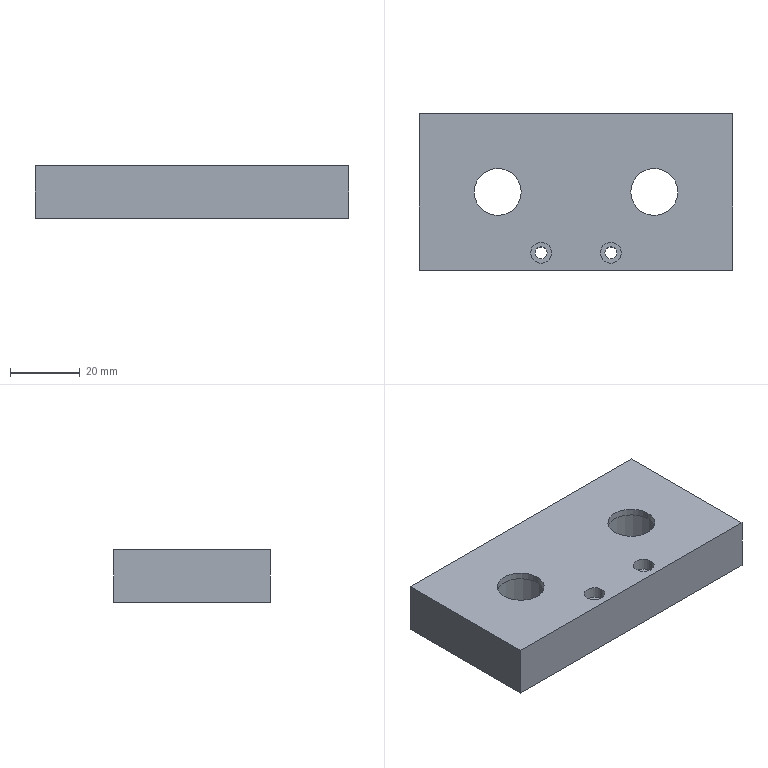Part | STEP file | X77-08308 | 1 solid | 26 faces | box 90 x 45 x 15 mm | volume 51606 mm3 | cylinder 16 | plane 10 | commonest cylinder face diameters 3.4 x4 6 x4 13.5 x4 20 x4
STEP:
#1=CARTESIAN_POINT('',(-591.701,750.64,11.6));
#2=VERTEX_POINT('',#1);
#3=CARTESIAN_POINT('',(-585.701,750.64,11.6));
#4=VERTEX_POINT('',#3);
#5=CARTESIAN_POINT('',(-588.701,750.64,11.6));
#6=DIRECTION('',(0.,0.,1.));
#7=DIRECTION('',(1.,0.,0.));
#8=AXIS2_PLACEMENT_3D('',#5,#6,#7);
#9=CIRCLE('',#8,3.);
#10=EDGE_CURVE('',#2,#4,#9,.T.);
#11=ORIENTED_EDGE('',*,*,#10,.F.);
#12=CARTESIAN_POINT('',(-591.701,750.64,15.));
#13=VERTEX_POINT('',#12);
#14=CARTESIAN_POINT('',(-591.701,750.64,15.));
#15=DIRECTION('',(0.,0.,1.));
#16=VECTOR('',#15,1000.);
#17=LINE('',#14,#16);
#18=EDGE_CURVE('',#2,#13,#17,.T.);
#19=ORIENTED_EDGE('',*,*,#18,.T.);
#20=CARTESIAN_POINT('',(-585.701,750.64,15.));
#21=VERTEX_POINT('',#20);
#22=CARTESIAN_POINT('',(-588.701,750.64,15.));
#23=DIRECTION('',(0.,0.,1.));
#24=DIRECTION('',(1.,0.,0.));
#25=AXIS2_PLACEMENT_3D('',#22,#23,#24);
#26=CIRCLE('',#25,3.);
#27=EDGE_CURVE('',#13,#21,#26,.T.);
#28=ORIENTED_EDGE('',*,*,#27,.T.);
#29=CARTESIAN_POINT('',(-585.701,750.64,15.));
#30=DIRECTION('',(0.,0.,1.));
#31=VECTOR('',#30,1000.);
#32=LINE('',#29,#31);
#33=EDGE_CURVE('',#4,#21,#32,.T.);
#34=ORIENTED_EDGE('',*,*,#33,.F.);
#35=EDGE_LOOP('',(#11,#19,#28,#34));
#36=FACE_OUTER_BOUND('',#35,.T.);
#37=CARTESIAN_POINT('',(-588.701,750.64,15.));
#38=DIRECTION('',(0.,0.,1.));
#39=DIRECTION('',(1.,0.,0.));
#40=AXIS2_PLACEMENT_3D('',#37,#38,#39);
#41=CYLINDRICAL_SURFACE('',#40,3.);
#42=ADVANCED_FACE('',(#36),#41,.F.);
#43=CARTESIAN_POINT('',(-590.401,750.64,0.));
#44=VERTEX_POINT('',#43);
#45=CARTESIAN_POINT('',(-587.001,750.64,0.));
#46=VERTEX_POINT('',#45);
#47=CARTESIAN_POINT('',(-588.701,750.64,0.));
#48=DIRECTION('',(0.,0.,1.));
#49=DIRECTION('',(1.,0.,0.));
#50=AXIS2_PLACEMENT_3D('',#47,#48,#49);
#51=CIRCLE('',#50,1.7);
#52=EDGE_CURVE('',#44,#46,#51,.T.);
#53=ORIENTED_EDGE('',*,*,#52,.F.);
#54=CARTESIAN_POINT('',(-590.401,750.64,11.6));
#55=VERTEX_POINT('',#54);
#56=CARTESIAN_POINT('',(-590.401,750.64,15.));
#57=DIRECTION('',(0.,0.,1.));
#58=VECTOR('',#57,1000.);
#59=LINE('',#56,#58);
#60=EDGE_CURVE('',#44,#55,#59,.T.);
#61=ORIENTED_EDGE('',*,*,#60,.T.);
#62=CARTESIAN_POINT('',(-587.001,750.64,11.6));
#63=VERTEX_POINT('',#62);
#64=CARTESIAN_POINT('',(-588.701,750.64,11.6));
#65=DIRECTION('',(0.,0.,1.));
#66=DIRECTION('',(1.,0.,0.));
#67=AXIS2_PLACEMENT_3D('',#64,#65,#66);
#68=CIRCLE('',#67,1.7);
#69=EDGE_CURVE('',#55,#63,#68,.T.);
#70=ORIENTED_EDGE('',*,*,#69,.T.);
#71=CARTESIAN_POINT('',(-587.001,750.64,15.));
#72=DIRECTION('',(0.,0.,1.));
#73=VECTOR('',#72,1000.);
#74=LINE('',#71,#73);
#75=EDGE_CURVE('',#46,#63,#74,.T.);
#76=ORIENTED_EDGE('',*,*,#75,.F.);
#77=EDGE_LOOP('',(#53,#61,#70,#76));
#78=FACE_OUTER_BOUND('',#77,.T.);
#79=CARTESIAN_POINT('',(-588.701,750.64,15.));
#80=DIRECTION('',(0.,0.,1.));
#81=DIRECTION('',(1.,0.,0.));
#82=AXIS2_PLACEMENT_3D('',#79,#80,#81);
#83=CYLINDRICAL_SURFACE('',#82,1.7);
#84=ADVANCED_FACE('',(#78),#83,.F.);
#85=CARTESIAN_POINT('',(-571.701,750.64,11.6));
#86=VERTEX_POINT('',#85);
#87=CARTESIAN_POINT('',(-565.701,750.64,11.6));
#88=VERTEX_POINT('',#87);
#89=CARTESIAN_POINT('',(-568.701,750.64,11.6));
#90=DIRECTION('',(0.,0.,1.));
#91=DIRECTION('',(1.,0.,0.));
#92=AXIS2_PLACEMENT_3D('',#89,#90,#91);
#93=CIRCLE('',#92,3.);
#94=EDGE_CURVE('',#86,#88,#93,.T.);
#95=ORIENTED_EDGE('',*,*,#94,.F.);
#96=CARTESIAN_POINT('',(-571.701,750.64,15.));
#97=VERTEX_POINT('',#96);
#98=CARTESIAN_POINT('',(-571.701,750.64,15.));
#99=DIRECTION('',(0.,0.,1.));
#100=VECTOR('',#99,1000.);
#101=LINE('',#98,#100);
#102=EDGE_CURVE('',#86,#97,#101,.T.);
#103=ORIENTED_EDGE('',*,*,#102,.T.);
#104=CARTESIAN_POINT('',(-565.701,750.64,15.));
#105=VERTEX_POINT('',#104);
#106=CARTESIAN_POINT('',(-568.701,750.64,15.));
#107=DIRECTION('',(0.,0.,1.));
#108=DIRECTION('',(1.,0.,0.));
#109=AXIS2_PLACEMENT_3D('',#106,#107,#108);
#110=CIRCLE('',#109,3.);
#111=EDGE_CURVE('',#97,#105,#110,.T.);
#112=ORIENTED_EDGE('',*,*,#111,.T.);
#113=CARTESIAN_POINT('',(-565.701,750.64,15.));
#114=DIRECTION('',(0.,0.,1.));
#115=VECTOR('',#114,1000.);
#116=LINE('',#113,#115);
#117=EDGE_CURVE('',#88,#105,#116,.T.);
#118=ORIENTED_EDGE('',*,*,#117,.F.);
#119=EDGE_LOOP('',(#95,#103,#112,#118));
#120=FACE_OUTER_BOUND('',#119,.T.);
#121=CARTESIAN_POINT('',(-568.701,750.64,15.));
#122=DIRECTION('',(0.,0.,1.));
#123=DIRECTION('',(1.,0.,0.));
#124=AXIS2_PLACEMENT_3D('',#121,#122,#123);
#125=CYLINDRICAL_SURFACE('',#124,3.);
#126=ADVANCED_FACE('',(#120),#125,.F.);
#127=CARTESIAN_POINT('',(-570.401,750.64,0.));
#128=VERTEX_POINT('',#127);
#129=CARTESIAN_POINT('',(-567.001,750.64,0.));
#130=VERTEX_POINT('',#129);
#131=CARTESIAN_POINT('',(-568.701,750.64,0.));
#132=DIRECTION('',(0.,0.,1.));
#133=DIRECTION('',(1.,0.,0.));
#134=AXIS2_PLACEMENT_3D('',#131,#132,#133);
#135=CIRCLE('',#134,1.7);
#136=EDGE_CURVE('',#128,#130,#135,.T.);
#137=ORIENTED_EDGE('',*,*,#136,.F.);
#138=CARTESIAN_POINT('',(-570.401,750.64,11.6));
#139=VERTEX_POINT('',#138);
#140=CARTESIAN_POINT('',(-570.401,750.64,15.));
#141=DIRECTION('',(0.,0.,1.));
#142=VECTOR('',#141,1000.);
#143=LINE('',#140,#142);
#144=EDGE_CURVE('',#128,#139,#143,.T.);
#145=ORIENTED_EDGE('',*,*,#144,.T.);
#146=CARTESIAN_POINT('',(-567.001,750.64,11.6));
#147=VERTEX_POINT('',#146);
#148=CARTESIAN_POINT('',(-568.701,750.64,11.6));
#149=DIRECTION('',(0.,0.,1.));
#150=DIRECTION('',(1.,0.,0.));
#151=AXIS2_PLACEMENT_3D('',#148,#149,#150);
#152=CIRCLE('',#151,1.7);
#153=EDGE_CURVE('',#139,#147,#152,.T.);
#154=ORIENTED_EDGE('',*,*,#153,.T.);
#155=CARTESIAN_POINT('',(-567.001,750.64,15.));
#156=DIRECTION('',(0.,0.,1.));
#157=VECTOR('',#156,1000.);
#158=LINE('',#155,#157);
#159=EDGE_CURVE('',#130,#147,#158,.T.);
#160=ORIENTED_EDGE('',*,*,#159,.F.);
#161=EDGE_LOOP('',(#137,#145,#154,#160));
#162=FACE_OUTER_BOUND('',#161,.T.);
#163=CARTESIAN_POINT('',(-568.701,750.64,15.));
#164=DIRECTION('',(0.,0.,1.));
#165=DIRECTION('',(1.,0.,0.));
#166=AXIS2_PLACEMENT_3D('',#163,#164,#165);
#167=CYLINDRICAL_SURFACE('',#166,1.7);
#168=ADVANCED_FACE('',(#162),#167,.F.);
#169=CARTESIAN_POINT('',(-546.201,768.14,13.));
#170=VERTEX_POINT('',#169);
#171=CARTESIAN_POINT('',(-566.201,768.14,13.));
#172=VERTEX_POINT('',#171);
#173=CARTESIAN_POINT('',(-556.201,768.14,13.));
#174=DIRECTION('',(0.,0.,-1.));
#175=DIRECTION('',(-1.,0.,0.));
#176=AXIS2_PLACEMENT_3D('',#173,#174,#175);
#177=CIRCLE('',#176,10.);
#178=EDGE_CURVE('',#170,#172,#177,.T.);
#179=ORIENTED_EDGE('',*,*,#178,.F.);
#180=CARTESIAN_POINT('',(-546.201,768.14,0.));
#181=VERTEX_POINT('',#180);
#182=CARTESIAN_POINT('',(-546.201,768.14,0.));
#183=DIRECTION('',(0.,0.,-1.));
#184=VECTOR('',#183,1000.);
#185=LINE('',#182,#184);
#186=EDGE_CURVE('',#170,#181,#185,.T.);
#187=ORIENTED_EDGE('',*,*,#186,.T.);
#188=CARTESIAN_POINT('',(-566.201,768.14,0.));
#189=VERTEX_POINT('',#188);
#190=CARTESIAN_POINT('',(-556.201,768.14,0.));
#191=DIRECTION('',(0.,0.,-1.));
#192=DIRECTION('',(-1.,0.,0.));
#193=AXIS2_PLACEMENT_3D('',#190,#191,#192);
#194=CIRCLE('',#193,10.);
#195=EDGE_CURVE('',#181,#189,#194,.T.);
#196=ORIENTED_EDGE('',*,*,#195,.T.);
#197=CARTESIAN_POINT('',(-566.201,768.14,0.));
#198=DIRECTION('',(0.,0.,-1.));
#199=VECTOR('',#198,1000.);
#200=LINE('',#197,#199);
#201=EDGE_CURVE('',#172,#189,#200,.T.);
#202=ORIENTED_EDGE('',*,*,#201,.F.);
#203=EDGE_LOOP('',(#179,#187,#196,#202));
#204=FACE_OUTER_BOUND('',#203,.T.);
#205=CARTESIAN_POINT('',(-556.201,768.14,0.));
#206=DIRECTION('',(0.,0.,-1.));
#207=DIRECTION('',(-1.,0.,0.));
#208=AXIS2_PLACEMENT_3D('',#205,#206,#207);
#209=CYLINDRICAL_SURFACE('',#208,10.);
#210=ADVANCED_FACE('',(#204),#209,.F.);
#211=CARTESIAN_POINT('',(-549.451,768.14,15.));
#212=VERTEX_POINT('',#211);
#213=CARTESIAN_POINT('',(-562.951,768.14,15.));
#214=VERTEX_POINT('',#213);
#215=CARTESIAN_POINT('',(-556.201,768.14,15.));
#216=DIRECTION('',(0.,0.,-1.));
#217=DIRECTION('',(-1.,0.,0.));
#218=AXIS2_PLACEMENT_3D('',#215,#216,#217);
#219=CIRCLE('',#218,6.75);
#220=EDGE_CURVE('',#212,#214,#219,.T.);
#221=ORIENTED_EDGE('',*,*,#220,.F.);
#222=CARTESIAN_POINT('',(-549.451,768.14,13.));
#223=VERTEX_POINT('',#222);
#224=CARTESIAN_POINT('',(-549.451,768.14,0.));
#225=DIRECTION('',(0.,0.,-1.));
#226=VECTOR('',#225,1000.);
#227=LINE('',#224,#226);
#228=EDGE_CURVE('',#212,#223,#227,.T.);
#229=ORIENTED_EDGE('',*,*,#228,.T.);
#230=CARTESIAN_POINT('',(-562.951,768.14,13.));
#231=VERTEX_POINT('',#230);
#232=CARTESIAN_POINT('',(-556.201,768.14,13.));
#233=DIRECTION('',(0.,0.,-1.));
#234=DIRECTION('',(-1.,0.,0.));
#235=AXIS2_PLACEMENT_3D('',#232,#233,#234);
#236=CIRCLE('',#235,6.75);
#237=EDGE_CURVE('',#223,#231,#236,.T.);
#238=ORIENTED_EDGE('',*,*,#237,.T.);
#239=CARTESIAN_POINT('',(-562.951,768.14,0.));
#240=DIRECTION('',(0.,0.,-1.));
#241=VECTOR('',#240,1000.);
#242=LINE('',#239,#241);
#243=EDGE_CURVE('',#214,#231,#242,.T.);
#244=ORIENTED_EDGE('',*,*,#243,.F.);
#245=EDGE_LOOP('',(#221,#229,#238,#244));
#246=FACE_OUTER_BOUND('',#245,.T.);
#247=CARTESIAN_POINT('',(-556.201,768.14,0.));
#248=DIRECTION('',(0.,0.,-1.));
#249=DIRECTION('',(-1.,0.,0.));
#250=AXIS2_PLACEMENT_3D('',#247,#248,#249);
#251=CYLINDRICAL_SURFACE('',#250,6.75);
#252=ADVANCED_FACE('',(#246),#251,.F.);
#253=CARTESIAN_POINT('',(-591.201,768.14,13.));
#254=VERTEX_POINT('',#253);
#255=CARTESIAN_POINT('',(-611.201,768.14,13.));
#256=VERTEX_POINT('',#255);
#257=CARTESIAN_POINT('',(-601.201,768.14,13.));
#258=DIRECTION('',(0.,0.,-1.));
#259=DIRECTION('',(-1.,0.,0.));
#260=AXIS2_PLACEMENT_3D('',#257,#258,#259);
#261=CIRCLE('',#260,10.);
#262=EDGE_CURVE('',#254,#256,#261,.T.);
#263=ORIENTED_EDGE('',*,*,#262,.F.);
#264=CARTESIAN_POINT('',(-591.201,768.14,0.));
#265=VERTEX_POINT('',#264);
#266=CARTESIAN_POINT('',(-591.201,768.14,0.));
#267=DIRECTION('',(0.,0.,-1.));
#268=VECTOR('',#267,1000.);
#269=LINE('',#266,#268);
#270=EDGE_CURVE('',#254,#265,#269,.T.);
#271=ORIENTED_EDGE('',*,*,#270,.T.);
#272=CARTESIAN_POINT('',(-611.201,768.14,0.));
#273=VERTEX_POINT('',#272);
#274=CARTESIAN_POINT('',(-601.201,768.14,0.));
#275=DIRECTION('',(0.,0.,-1.));
#276=DIRECTION('',(-1.,0.,0.));
#277=AXIS2_PLACEMENT_3D('',#274,#275,#276);
#278=CIRCLE('',#277,10.);
#279=EDGE_CURVE('',#265,#273,#278,.T.);
#280=ORIENTED_EDGE('',*,*,#279,.T.);
#281=CARTESIAN_POINT('',(-611.201,768.14,0.));
#282=DIRECTION('',(0.,0.,-1.));
#283=VECTOR('',#282,1000.);
#284=LINE('',#281,#283);
#285=EDGE_CURVE('',#256,#273,#284,.T.);
#286=ORIENTED_EDGE('',*,*,#285,.F.);
#287=EDGE_LOOP('',(#263,#271,#280,#286));
#288=FACE_OUTER_BOUND('',#287,.T.);
#289=CARTESIAN_POINT('',(-601.201,768.14,0.));
#290=DIRECTION('',(0.,0.,-1.));
#291=DIRECTION('',(-1.,0.,0.));
#292=AXIS2_PLACEMENT_3D('',#289,#290,#291);
#293=CYLINDRICAL_SURFACE('',#292,10.);
#294=ADVANCED_FACE('',(#288),#293,.F.);
#295=CARTESIAN_POINT('',(-594.451,768.14,15.));
#296=VERTEX_POINT('',#295);
#297=CARTESIAN_POINT('',(-607.951,768.14,15.));
#298=VERTEX_POINT('',#297);
#299=CARTESIAN_POINT('',(-601.201,768.14,15.));
#300=DIRECTION('',(0.,0.,-1.));
#301=DIRECTION('',(-1.,0.,0.));
#302=AXIS2_PLACEMENT_3D('',#299,#300,#301);
#303=CIRCLE('',#302,6.75);
#304=EDGE_CURVE('',#296,#298,#303,.T.);
#305=ORIENTED_EDGE('',*,*,#304,.F.);
#306=CARTESIAN_POINT('',(-594.451,768.14,13.));
#307=VERTEX_POINT('',#306);
#308=CARTESIAN_POINT('',(-594.451,768.14,0.));
#309=DIRECTION('',(0.,0.,-1.));
#310=VECTOR('',#309,1000.);
#311=LINE('',#308,#310);
#312=EDGE_CURVE('',#296,#307,#311,.T.);
#313=ORIENTED_EDGE('',*,*,#312,.T.);
#314=CARTESIAN_POINT('',(-607.951,768.14,13.));
#315=VERTEX_POINT('',#314);
#316=CARTESIAN_POINT('',(-601.201,768.14,13.));
#317=DIRECTION('',(0.,0.,-1.));
#318=DIRECTION('',(-1.,0.,0.));
#319=AXIS2_PLACEMENT_3D('',#316,#317,#318);
#320=CIRCLE('',#319,6.75);
#321=EDGE_CURVE('',#307,#315,#320,.T.);
#322=ORIENTED_EDGE('',*,*,#321,.T.);
#323=CARTESIAN_POINT('',(-607.951,768.14,0.));
#324=DIRECTION('',(0.,0.,-1.));
#325=VECTOR('',#324,1000.);
#326=LINE('',#323,#325);
#327=EDGE_CURVE('',#298,#315,#326,.T.);
#328=ORIENTED_EDGE('',*,*,#327,.F.);
#329=EDGE_LOOP('',(#305,#313,#322,#328));
#330=FACE_OUTER_BOUND('',#329,.T.);
#331=CARTESIAN_POINT('',(-601.201,768.14,0.));
#332=DIRECTION('',(0.,0.,-1.));
#333=DIRECTION('',(-1.,0.,0.));
#334=AXIS2_PLACEMENT_3D('',#331,#332,#333);
#335=CYLINDRICAL_SURFACE('',#334,6.75);
#336=ADVANCED_FACE('',(#330),#335,.F.);
#337=CARTESIAN_POINT('',(-623.701,790.64,0.));
#338=VERTEX_POINT('',#337);
#339=CARTESIAN_POINT('',(-623.701,745.64,0.));
#340=VERTEX_POINT('',#339);
#341=CARTESIAN_POINT('',(-623.701,790.64,0.));
#342=DIRECTION('',(0.,-1.,0.));
#343=VECTOR('',#342,1000.);
#344=LINE('',#341,#343);
#345=EDGE_CURVE('',#338,#340,#344,.T.);
#346=ORIENTED_EDGE('',*,*,#345,.T.);
#347=CARTESIAN_POINT('',(-623.701,745.64,15.));
#348=VERTEX_POINT('',#347);
#349=CARTESIAN_POINT('',(-623.701,745.64,15.));
#350=DIRECTION('',(0.,0.,-1.));
#351=VECTOR('',#350,1000.);
#352=LINE('',#349,#351);
#353=EDGE_CURVE('',#348,#340,#352,.T.);
#354=ORIENTED_EDGE('',*,*,#353,.F.);
#355=CARTESIAN_POINT('',(-623.701,790.64,15.));
#356=VERTEX_POINT('',#355);
#357=CARTESIAN_POINT('',(-623.701,790.64,15.));
#358=DIRECTION('',(0.,-1.,0.));
#359=VECTOR('',#358,1000.);
#360=LINE('',#357,#359);
#361=EDGE_CURVE('',#356,#348,#360,.T.);
#362=ORIENTED_EDGE('',*,*,#361,.F.);
#363=CARTESIAN_POINT('',(-623.701,790.64,15.));
#364=DIRECTION('',(0.,0.,-1.));
#365=VECTOR('',#364,1000.);
#366=LINE('',#363,#365);
#367=EDGE_CURVE('',#356,#338,#366,.T.);
#368=ORIENTED_EDGE('',*,*,#367,.T.);
#369=EDGE_LOOP('',(#346,#354,#362,#368));
#370=FACE_OUTER_BOUND('',#369,.T.);
#371=CARTESIAN_POINT('',(-623.701,790.64,15.));
#372=DIRECTION('',(1.,0.,0.));
#373=DIRECTION('',(0.,0.,-1.));
#374=AXIS2_PLACEMENT_3D('',#371,#372,#373);
#375=PLANE('',#374);
#376=ADVANCED_FACE('',(#370),#375,.F.);
#377=CARTESIAN_POINT('',(-533.701,745.64,0.));
#378=VERTEX_POINT('',#377);
#379=CARTESIAN_POINT('',(-623.701,745.64,0.));
#380=DIRECTION('',(1.,0.,0.));
#381=VECTOR('',#380,1000.);
#382=LINE('',#379,#381);
#383=EDGE_CURVE('',#340,#378,#382,.T.);
#384=ORIENTED_EDGE('',*,*,#383,.T.);
#385=CARTESIAN_POINT('',(-533.701,745.64,15.));
#386=VERTEX_POINT('',#385);
#387=CARTESIAN_POINT('',(-533.701,745.64,15.));
#388=DIRECTION('',(0.,0.,-1.));
#389=VECTOR('',#388,1000.);
#390=LINE('',#387,#389);
#391=EDGE_CURVE('',#386,#378,#390,.T.);
#392=ORIENTED_EDGE('',*,*,#391,.F.);
#393=CARTESIAN_POINT('',(-623.701,745.64,15.));
#394=DIRECTION('',(1.,0.,0.));
#395=VECTOR('',#394,1000.);
#396=LINE('',#393,#395);
#397=EDGE_CURVE('',#348,#386,#396,.T.);
#398=ORIENTED_EDGE('',*,*,#397,.F.);
#399=ORIENTED_EDGE('',*,*,#353,.T.);
#400=EDGE_LOOP('',(#384,#392,#398,#399));
#401=FACE_OUTER_BOUND('',#400,.T.);
#402=CARTESIAN_POINT('',(-623.701,745.64,15.));
#403=DIRECTION('',(0.,1.,0.));
#404=DIRECTION('',(0.,0.,1.));
#405=AXIS2_PLACEMENT_3D('',#402,#403,#404);
#406=PLANE('',#405);
#407=ADVANCED_FACE('',(#401),#406,.F.);
#408=CARTESIAN_POINT('',(-533.701,790.64,0.));
#409=VERTEX_POINT('',#408);
#410=CARTESIAN_POINT('',(-533.701,790.64,0.));
#411=DIRECTION('',(0.,1.,0.));
#412=VECTOR('',#411,1000.);
#413=LINE('',#410,#412);
#414=EDGE_CURVE('',#378,#409,#413,.T.);
#415=ORIENTED_EDGE('',*,*,#414,.T.);
#416=CARTESIAN_POINT('',(-533.701,790.64,15.));
#417=VERTEX_POINT('',#416);
#418=CARTESIAN_POINT('',(-533.701,790.64,15.));
#419=DIRECTION('',(0.,0.,-1.));
#420=VECTOR('',#419,1000.);
#421=LINE('',#418,#420);
#422=EDGE_CURVE('',#417,#409,#421,.T.);
#423=ORIENTED_EDGE('',*,*,#422,.F.);
#424=CARTESIAN_POINT('',(-533.701,790.64,15.));
#425=DIRECTION('',(0.,1.,0.));
#426=VECTOR('',#425,1000.);
#427=LINE('',#424,#426);
#428=EDGE_CURVE('',#386,#417,#427,.T.);
#429=ORIENTED_EDGE('',*,*,#428,.F.);
#430=ORIENTED_EDGE('',*,*,#391,.T.);
#431=EDGE_LOOP('',(#415,#423,#429,#430));
#432=FACE_OUTER_BOUND('',#431,.T.);
#433=CARTESIAN_POINT('',(-533.701,790.64,15.));
#434=DIRECTION('',(-1.,0.,0.));
#435=DIRECTION('',(0.,0.,1.));
#436=AXIS2_PLACEMENT_3D('',#433,#434,#435);
#437=PLANE('',#436);
#438=ADVANCED_FACE('',(#432),#437,.F.);
#439=CARTESIAN_POINT('',(-623.701,790.64,0.));
#440=DIRECTION('',(-1.,0.,0.));
#441=VECTOR('',#440,1000.);
#442=LINE('',#439,#441);
#443=EDGE_CURVE('',#409,#338,#442,.T.);
#444=ORIENTED_EDGE('',*,*,#443,.T.);
#445=ORIENTED_EDGE('',*,*,#367,.F.);
#446=CARTESIAN_POINT('',(-623.701,790.64,15.));
#447=DIRECTION('',(-1.,0.,0.));
#448=VECTOR('',#447,1000.);
#449=LINE('',#446,#448);
#450=EDGE_CURVE('',#417,#356,#449,.T.);
#451=ORIENTED_EDGE('',*,*,#450,.F.);
#452=ORIENTED_EDGE('',*,*,#422,.T.);
#453=EDGE_LOOP('',(#444,#445,#451,#452));
#454=FACE_OUTER_BOUND('',#453,.T.);
#455=CARTESIAN_POINT('',(-623.701,790.64,15.));
#456=DIRECTION('',(0.,-1.,0.));
#457=DIRECTION('',(0.,0.,-1.));
#458=AXIS2_PLACEMENT_3D('',#455,#456,#457);
#459=PLANE('',#458);
#460=ADVANCED_FACE('',(#454),#459,.F.);
#461=CARTESIAN_POINT('',(-588.701,750.64,15.));
#462=DIRECTION('',(0.,0.,1.));
#463=DIRECTION('',(1.,0.,0.));
#464=AXIS2_PLACEMENT_3D('',#461,#462,#463);
#465=CIRCLE('',#464,3.);
#466=EDGE_CURVE('',#21,#13,#465,.T.);
#467=ORIENTED_EDGE('',*,*,#466,.F.);
#468=ORIENTED_EDGE('',*,*,#27,.F.);
#469=EDGE_LOOP('',(#467,#468));
#470=FACE_BOUND('',#469,.T.);
#471=CARTESIAN_POINT('',(-568.701,750.64,15.));
#472=DIRECTION('',(0.,0.,1.));
#473=DIRECTION('',(1.,0.,0.));
#474=AXIS2_PLACEMENT_3D('',#471,#472,#473);
#475=CIRCLE('',#474,3.);
#476=EDGE_CURVE('',#105,#97,#475,.T.);
#477=ORIENTED_EDGE('',*,*,#476,.F.);
#478=ORIENTED_EDGE('',*,*,#111,.F.);
#479=EDGE_LOOP('',(#477,#478));
#480=FACE_BOUND('',#479,.T.);
#481=CARTESIAN_POINT('',(-556.201,768.14,15.));
#482=DIRECTION('',(0.,0.,-1.));
#483=DIRECTION('',(-1.,0.,0.));
#484=AXIS2_PLACEMENT_3D('',#481,#482,#483);
#485=CIRCLE('',#484,6.75);
#486=EDGE_CURVE('',#214,#212,#485,.T.);
#487=ORIENTED_EDGE('',*,*,#486,.T.);
#488=ORIENTED_EDGE('',*,*,#220,.T.);
#489=EDGE_LOOP('',(#487,#488));
#490=FACE_BOUND('',#489,.T.);
#491=CARTESIAN_POINT('',(-601.201,768.14,15.));
#492=DIRECTION('',(0.,0.,-1.));
#493=DIRECTION('',(-1.,0.,0.));
#494=AXIS2_PLACEMENT_3D('',#491,#492,#493);
#495=CIRCLE('',#494,6.75);
#496=EDGE_CURVE('',#298,#296,#495,.T.);
#497=ORIENTED_EDGE('',*,*,#496,.T.);
#498=ORIENTED_EDGE('',*,*,#304,.T.);
#499=EDGE_LOOP('',(#497,#498));
#500=FACE_BOUND('',#499,.T.);
#501=ORIENTED_EDGE('',*,*,#361,.T.);
#502=ORIENTED_EDGE('',*,*,#397,.T.);
#503=ORIENTED_EDGE('',*,*,#428,.T.);
#504=ORIENTED_EDGE('',*,*,#450,.T.);
#505=EDGE_LOOP('',(#501,#502,#503,#504));
#506=FACE_OUTER_BOUND('',#505,.T.);
#507=CARTESIAN_POINT('',(-623.701,745.64,15.));
#508=DIRECTION('',(0.,0.,1.));
#509=DIRECTION('',(1.,0.,0.));
#510=AXIS2_PLACEMENT_3D('',#507,#508,#509);
#511=PLANE('',#510);
#512=ADVANCED_FACE('',(#470,#480,#490,#500,#506),#511,.T.);
#513=CARTESIAN_POINT('',(-588.701,750.64,0.));
#514=DIRECTION('',(0.,0.,1.));
#515=DIRECTION('',(1.,0.,0.));
#516=AXIS2_PLACEMENT_3D('',#513,#514,#515);
#517=CIRCLE('',#516,1.7);
#518=EDGE_CURVE('',#46,#44,#517,.T.);
#519=ORIENTED_EDGE('',*,*,#518,.T.);
#520=ORIENTED_EDGE('',*,*,#52,.T.);
#521=EDGE_LOOP('',(#519,#520));
#522=FACE_BOUND('',#521,.T.);
#523=CARTESIAN_POINT('',(-568.701,750.64,0.));
#524=DIRECTION('',(0.,0.,1.));
#525=DIRECTION('',(1.,0.,0.));
#526=AXIS2_PLACEMENT_3D('',#523,#524,#525);
#527=CIRCLE('',#526,1.7);
#528=EDGE_CURVE('',#130,#128,#527,.T.);
#529=ORIENTED_EDGE('',*,*,#528,.T.);
#530=ORIENTED_EDGE('',*,*,#136,.T.);
#531=EDGE_LOOP('',(#529,#530));
#532=FACE_BOUND('',#531,.T.);
#533=CARTESIAN_POINT('',(-556.201,768.14,0.));
#534=DIRECTION('',(0.,0.,-1.));
#535=DIRECTION('',(-1.,0.,0.));
#536=AXIS2_PLACEMENT_3D('',#533,#534,#535);
#537=CIRCLE('',#536,10.);
#538=EDGE_CURVE('',#189,#181,#537,.T.);
#539=ORIENTED_EDGE('',*,*,#538,.F.);
#540=ORIENTED_EDGE('',*,*,#195,.F.);
#541=EDGE_LOOP('',(#539,#540));
#542=FACE_BOUND('',#541,.T.);
#543=CARTESIAN_POINT('',(-601.201,768.14,0.));
#544=DIRECTION('',(0.,0.,-1.));
#545=DIRECTION('',(-1.,0.,0.));
#546=AXIS2_PLACEMENT_3D('',#543,#544,#545);
#547=CIRCLE('',#546,10.);
#548=EDGE_CURVE('',#273,#265,#547,.T.);
#549=ORIENTED_EDGE('',*,*,#548,.F.);
#550=ORIENTED_EDGE('',*,*,#279,.F.);
#551=EDGE_LOOP('',(#549,#550));
#552=FACE_BOUND('',#551,.T.);
#553=ORIENTED_EDGE('',*,*,#345,.F.);
#554=ORIENTED_EDGE('',*,*,#443,.F.);
#555=ORIENTED_EDGE('',*,*,#414,.F.);
#556=ORIENTED_EDGE('',*,*,#383,.F.);
#557=EDGE_LOOP('',(#553,#554,#555,#556));
#558=FACE_OUTER_BOUND('',#557,.T.);
#559=CARTESIAN_POINT('',(-623.701,745.64,0.));
#560=DIRECTION('',(0.,0.,1.));
#561=DIRECTION('',(1.,0.,0.));
#562=AXIS2_PLACEMENT_3D('',#559,#560,#561);
#563=PLANE('',#562);
#564=ADVANCED_FACE('',(#522,#532,#542,#552,#558),#563,.F.);
#565=ORIENTED_EDGE('',*,*,#312,.F.);
#566=ORIENTED_EDGE('',*,*,#496,.F.);
#567=ORIENTED_EDGE('',*,*,#327,.T.);
#568=CARTESIAN_POINT('',(-601.201,768.14,13.));
#569=DIRECTION('',(0.,0.,-1.));
#570=DIRECTION('',(-1.,0.,0.));
#571=AXIS2_PLACEMENT_3D('',#568,#569,#570);
#572=CIRCLE('',#571,6.75);
#573=EDGE_CURVE('',#315,#307,#572,.T.);
#574=ORIENTED_EDGE('',*,*,#573,.T.);
#575=EDGE_LOOP('',(#565,#566,#567,#574));
#576=FACE_OUTER_BOUND('',#575,.T.);
#577=CARTESIAN_POINT('',(-601.201,768.14,0.));
#578=DIRECTION('',(0.,0.,-1.));
#579=DIRECTION('',(-1.,0.,0.));
#580=AXIS2_PLACEMENT_3D('',#577,#578,#579);
#581=CYLINDRICAL_SURFACE('',#580,6.75);
#582=ADVANCED_FACE('',(#576),#581,.F.);
#583=ORIENTED_EDGE('',*,*,#573,.F.);
#584=ORIENTED_EDGE('',*,*,#321,.F.);
#585=EDGE_LOOP('',(#583,#584));
#586=FACE_BOUND('',#585,.T.);
#587=CARTESIAN_POINT('',(-601.201,768.14,13.));
#588=DIRECTION('',(0.,0.,-1.));
#589=DIRECTION('',(-1.,0.,0.));
#590=AXIS2_PLACEMENT_3D('',#587,#588,#589);
#591=CIRCLE('',#590,10.);
#592=EDGE_CURVE('',#256,#254,#591,.T.);
#593=ORIENTED_EDGE('',*,*,#592,.T.);
#594=ORIENTED_EDGE('',*,*,#262,.T.);
#595=EDGE_LOOP('',(#593,#594));
#596=FACE_OUTER_BOUND('',#595,.T.);
#597=CARTESIAN_POINT('',(-594.451,768.14,13.));
#598=DIRECTION('',(0.,0.,1.));
#599=DIRECTION('',(1.,0.,0.));
#600=AXIS2_PLACEMENT_3D('',#597,#598,#599);
#601=PLANE('',#600);
#602=ADVANCED_FACE('',(#586,#596),#601,.F.);
#603=ORIENTED_EDGE('',*,*,#270,.F.);
#604=ORIENTED_EDGE('',*,*,#592,.F.);
#605=ORIENTED_EDGE('',*,*,#285,.T.);
#606=ORIENTED_EDGE('',*,*,#548,.T.);
#607=EDGE_LOOP('',(#603,#604,#605,#606));
#608=FACE_OUTER_BOUND('',#607,.T.);
#609=CARTESIAN_POINT('',(-601.201,768.14,0.));
#610=DIRECTION('',(0.,0.,-1.));
#611=DIRECTION('',(-1.,0.,0.));
#612=AXIS2_PLACEMENT_3D('',#609,#610,#611);
#613=CYLINDRICAL_SURFACE('',#612,10.);
#614=ADVANCED_FACE('',(#608),#613,.F.);
#615=ORIENTED_EDGE('',*,*,#228,.F.);
#616=ORIENTED_EDGE('',*,*,#486,.F.);
#617=ORIENTED_EDGE('',*,*,#243,.T.);
#618=CARTESIAN_POINT('',(-556.201,768.14,13.));
#619=DIRECTION('',(0.,0.,-1.));
#620=DIRECTION('',(-1.,0.,0.));
#621=AXIS2_PLACEMENT_3D('',#618,#619,#620);
#622=CIRCLE('',#621,6.75);
#623=EDGE_CURVE('',#231,#223,#622,.T.);
#624=ORIENTED_EDGE('',*,*,#623,.T.);
#625=EDGE_LOOP('',(#615,#616,#617,#624));
#626=FACE_OUTER_BOUND('',#625,.T.);
#627=CARTESIAN_POINT('',(-556.201,768.14,0.));
#628=DIRECTION('',(0.,0.,-1.));
#629=DIRECTION('',(-1.,0.,0.));
#630=AXIS2_PLACEMENT_3D('',#627,#628,#629);
#631=CYLINDRICAL_SURFACE('',#630,6.75);
#632=ADVANCED_FACE('',(#626),#631,.F.);
#633=ORIENTED_EDGE('',*,*,#623,.F.);
#634=ORIENTED_EDGE('',*,*,#237,.F.);
#635=EDGE_LOOP('',(#633,#634));
#636=FACE_BOUND('',#635,.T.);
#637=CARTESIAN_POINT('',(-556.201,768.14,13.));
#638=DIRECTION('',(0.,0.,-1.));
#639=DIRECTION('',(-1.,0.,0.));
#640=AXIS2_PLACEMENT_3D('',#637,#638,#639);
#641=CIRCLE('',#640,10.);
#642=EDGE_CURVE('',#172,#170,#641,.T.);
#643=ORIENTED_EDGE('',*,*,#642,.T.);
#644=ORIENTED_EDGE('',*,*,#178,.T.);
#645=EDGE_LOOP('',(#643,#644));
#646=FACE_OUTER_BOUND('',#645,.T.);
#647=CARTESIAN_POINT('',(-549.451,768.14,13.));
#648=DIRECTION('',(0.,0.,1.));
#649=DIRECTION('',(1.,0.,0.));
#650=AXIS2_PLACEMENT_3D('',#647,#648,#649);
#651=PLANE('',#650);
#652=ADVANCED_FACE('',(#636,#646),#651,.F.);
#653=ORIENTED_EDGE('',*,*,#186,.F.);
#654=ORIENTED_EDGE('',*,*,#642,.F.);
#655=ORIENTED_EDGE('',*,*,#201,.T.);
#656=ORIENTED_EDGE('',*,*,#538,.T.);
#657=EDGE_LOOP('',(#653,#654,#655,#656));
#658=FACE_OUTER_BOUND('',#657,.T.);
#659=CARTESIAN_POINT('',(-556.201,768.14,0.));
#660=DIRECTION('',(0.,0.,-1.));
#661=DIRECTION('',(-1.,0.,0.));
#662=AXIS2_PLACEMENT_3D('',#659,#660,#661);
#663=CYLINDRICAL_SURFACE('',#662,10.);
#664=ADVANCED_FACE('',(#658),#663,.F.);
#665=ORIENTED_EDGE('',*,*,#144,.F.);
#666=ORIENTED_EDGE('',*,*,#528,.F.);
#667=ORIENTED_EDGE('',*,*,#159,.T.);
#668=CARTESIAN_POINT('',(-568.701,750.64,11.6));
#669=DIRECTION('',(0.,0.,1.));
#670=DIRECTION('',(1.,0.,0.));
#671=AXIS2_PLACEMENT_3D('',#668,#669,#670);
#672=CIRCLE('',#671,1.7);
#673=EDGE_CURVE('',#147,#139,#672,.T.);
#674=ORIENTED_EDGE('',*,*,#673,.T.);
#675=EDGE_LOOP('',(#665,#666,#667,#674));
#676=FACE_OUTER_BOUND('',#675,.T.);
#677=CARTESIAN_POINT('',(-568.701,750.64,15.));
#678=DIRECTION('',(0.,0.,1.));
#679=DIRECTION('',(1.,0.,0.));
#680=AXIS2_PLACEMENT_3D('',#677,#678,#679);
#681=CYLINDRICAL_SURFACE('',#680,1.7);
#682=ADVANCED_FACE('',(#676),#681,.F.);
#683=ORIENTED_EDGE('',*,*,#673,.F.);
#684=ORIENTED_EDGE('',*,*,#153,.F.);
#685=EDGE_LOOP('',(#683,#684));
#686=FACE_BOUND('',#685,.T.);
#687=CARTESIAN_POINT('',(-568.701,750.64,11.6));
#688=DIRECTION('',(0.,0.,1.));
#689=DIRECTION('',(1.,0.,0.));
#690=AXIS2_PLACEMENT_3D('',#687,#688,#689);
#691=CIRCLE('',#690,3.);
#692=EDGE_CURVE('',#88,#86,#691,.T.);
#693=ORIENTED_EDGE('',*,*,#692,.T.);
#694=ORIENTED_EDGE('',*,*,#94,.T.);
#695=EDGE_LOOP('',(#693,#694));
#696=FACE_OUTER_BOUND('',#695,.T.);
#697=CARTESIAN_POINT('',(-567.001,750.64,11.6));
#698=DIRECTION('',(0.,0.,-1.));
#699=DIRECTION('',(-1.,0.,0.));
#700=AXIS2_PLACEMENT_3D('',#697,#698,#699);
#701=PLANE('',#700);
#702=ADVANCED_FACE('',(#686,#696),#701,.F.);
#703=ORIENTED_EDGE('',*,*,#102,.F.);
#704=ORIENTED_EDGE('',*,*,#692,.F.);
#705=ORIENTED_EDGE('',*,*,#117,.T.);
#706=ORIENTED_EDGE('',*,*,#476,.T.);
#707=EDGE_LOOP('',(#703,#704,#705,#706));
#708=FACE_OUTER_BOUND('',#707,.T.);
#709=CARTESIAN_POINT('',(-568.701,750.64,15.));
#710=DIRECTION('',(0.,0.,1.));
#711=DIRECTION('',(1.,0.,0.));
#712=AXIS2_PLACEMENT_3D('',#709,#710,#711);
#713=CYLINDRICAL_SURFACE('',#712,3.);
#714=ADVANCED_FACE('',(#708),#713,.F.);
#715=ORIENTED_EDGE('',*,*,#60,.F.);
#716=ORIENTED_EDGE('',*,*,#518,.F.);
#717=ORIENTED_EDGE('',*,*,#75,.T.);
#718=CARTESIAN_POINT('',(-588.701,750.64,11.6));
#719=DIRECTION('',(0.,0.,1.));
#720=DIRECTION('',(1.,0.,0.));
#721=AXIS2_PLACEMENT_3D('',#718,#719,#720);
#722=CIRCLE('',#721,1.7);
#723=EDGE_CURVE('',#63,#55,#722,.T.);
#724=ORIENTED_EDGE('',*,*,#723,.T.);
#725=EDGE_LOOP('',(#715,#716,#717,#724));
#726=FACE_OUTER_BOUND('',#725,.T.);
#727=CARTESIAN_POINT('',(-588.701,750.64,15.));
#728=DIRECTION('',(0.,0.,1.));
#729=DIRECTION('',(1.,0.,0.));
#730=AXIS2_PLACEMENT_3D('',#727,#728,#729);
#731=CYLINDRICAL_SURFACE('',#730,1.7);
#732=ADVANCED_FACE('',(#726),#731,.F.);
#733=ORIENTED_EDGE('',*,*,#723,.F.);
#734=ORIENTED_EDGE('',*,*,#69,.F.);
#735=EDGE_LOOP('',(#733,#734));
#736=FACE_BOUND('',#735,.T.);
#737=CARTESIAN_POINT('',(-588.701,750.64,11.6));
#738=DIRECTION('',(0.,0.,1.));
#739=DIRECTION('',(1.,0.,0.));
#740=AXIS2_PLACEMENT_3D('',#737,#738,#739);
#741=CIRCLE('',#740,3.);
#742=EDGE_CURVE('',#4,#2,#741,.T.);
#743=ORIENTED_EDGE('',*,*,#742,.T.);
#744=ORIENTED_EDGE('',*,*,#10,.T.);
#745=EDGE_LOOP('',(#743,#744));
#746=FACE_OUTER_BOUND('',#745,.T.);
#747=CARTESIAN_POINT('',(-587.001,750.64,11.6));
#748=DIRECTION('',(0.,0.,-1.));
#749=DIRECTION('',(-1.,0.,0.));
#750=AXIS2_PLACEMENT_3D('',#747,#748,#749);
#751=PLANE('',#750);
#752=ADVANCED_FACE('',(#736,#746),#751,.F.);
#753=ORIENTED_EDGE('',*,*,#18,.F.);
#754=ORIENTED_EDGE('',*,*,#742,.F.);
#755=ORIENTED_EDGE('',*,*,#33,.T.);
#756=ORIENTED_EDGE('',*,*,#466,.T.);
#757=EDGE_LOOP('',(#753,#754,#755,#756));
#758=FACE_OUTER_BOUND('',#757,.T.);
#759=CARTESIAN_POINT('',(-588.701,750.64,15.));
#760=DIRECTION('',(0.,0.,1.));
#761=DIRECTION('',(1.,0.,0.));
#762=AXIS2_PLACEMENT_3D('',#759,#760,#761);
#763=CYLINDRICAL_SURFACE('',#762,3.);
#764=ADVANCED_FACE('',(#758),#763,.F.);
#765=CLOSED_SHELL('',(#42,#84,#126,#168,#210,#252,#294,#336,#376,#407,#438,#460,#512,#564,#582,#602,#614,#632,#652,#664,#682,#702,#714,#732,#752,#764));
#766=MANIFOLD_SOLID_BREP('',#765);
#767=CARTESIAN_POINT('',(0.,0.,0.));
#768=DIRECTION('',(0.,0.,1.));
#769=DIRECTION('',(1.,0.,0.));
#770=AXIS2_PLACEMENT_3D('',#767,#768,#769);
#771=(LENGTH_UNIT()NAMED_UNIT(*)SI_UNIT(.MILLI.,.METRE.));
#772=UNCERTAINTY_MEASURE_WITH_UNIT(LENGTH_MEASURE(0.00001),#771,'','');
#773=(NAMED_UNIT(*)PLANE_ANGLE_UNIT()SI_UNIT($,.RADIAN.));
#774=(NAMED_UNIT(*)SI_UNIT($,.STERADIAN.)SOLID_ANGLE_UNIT());
#775=(GEOMETRIC_REPRESENTATION_CONTEXT(3)GLOBAL_UNCERTAINTY_ASSIGNED_CONTEXT((#772))GLOBAL_UNIT_ASSIGNED_CONTEXT((#771,#773,#774))REPRESENTATION_CONTEXT('',''));
#776=ADVANCED_BREP_SHAPE_REPRESENTATION('',(#766,#770),#775);